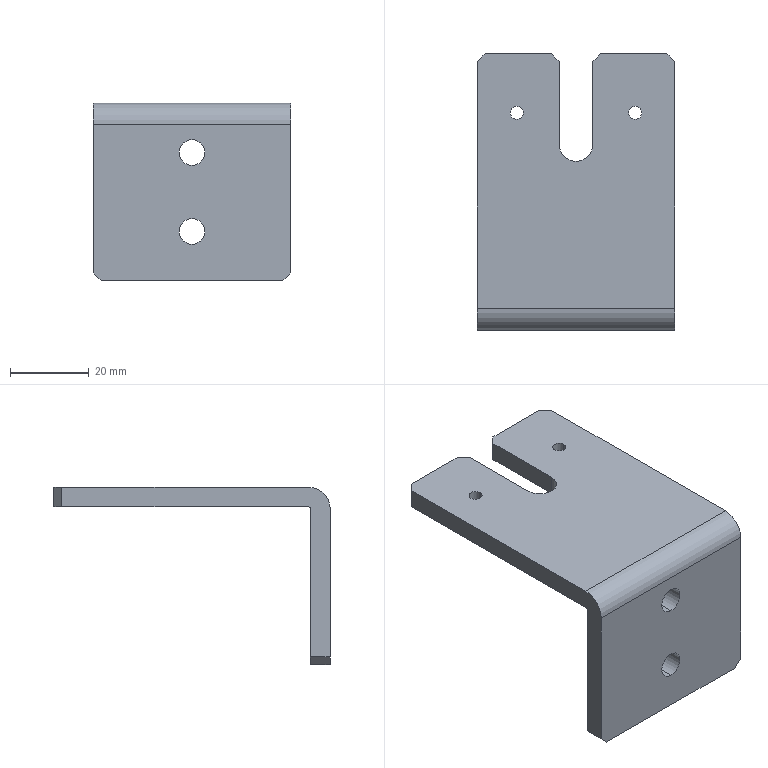Part | SolidWorks | features BaseBody 1 | 1 solid | 28 faces | box 50 x 70 x 45 mm | volume 25581 mm3 | plane 17 | cylinder 11 | commonest cylinder face diameters 3.3 x4 6.5 x4 1 x1 8.5 x1 11 x1
STEP:
#1=CARTESIAN_POINT('',(13.35,55.,-5.));
#2=VERTEX_POINT('',#1);
#3=CARTESIAN_POINT('',(16.65,55.,-5.));
#4=VERTEX_POINT('',#3);
#5=CARTESIAN_POINT('',(15.,55.,-5.));
#6=DIRECTION('',(0.,0.,1.));
#7=DIRECTION('',(1.,0.,0.));
#8=AXIS2_PLACEMENT_3D('',#5,#6,#7);
#9=CIRCLE('',#8,1.65);
#10=EDGE_CURVE('',#2,#4,#9,.T.);
#11=ORIENTED_EDGE('',*,*,#10,.F.);
#12=CARTESIAN_POINT('',(13.35,55.,0.));
#13=VERTEX_POINT('',#12);
#14=CARTESIAN_POINT('',(13.35,55.,0.));
#15=DIRECTION('',(0.,0.,1.));
#16=VECTOR('',#15,1000.);
#17=LINE('',#14,#16);
#18=EDGE_CURVE('',#2,#13,#17,.T.);
#19=ORIENTED_EDGE('',*,*,#18,.T.);
#20=CARTESIAN_POINT('',(16.65,55.,0.));
#21=VERTEX_POINT('',#20);
#22=CARTESIAN_POINT('',(15.,55.,0.));
#23=DIRECTION('',(0.,0.,-1.));
#24=DIRECTION('',(1.,0.,0.));
#25=AXIS2_PLACEMENT_3D('',#22,#23,#24);
#26=CIRCLE('',#25,1.65);
#27=EDGE_CURVE('',#21,#13,#26,.T.);
#28=ORIENTED_EDGE('',*,*,#27,.F.);
#29=CARTESIAN_POINT('',(16.65,55.,0.));
#30=DIRECTION('',(0.,0.,1.));
#31=VECTOR('',#30,1000.);
#32=LINE('',#29,#31);
#33=EDGE_CURVE('',#4,#21,#32,.T.);
#34=ORIENTED_EDGE('',*,*,#33,.F.);
#35=EDGE_LOOP('',(#11,#19,#28,#34));
#36=FACE_OUTER_BOUND('',#35,.T.);
#37=CARTESIAN_POINT('',(15.,55.,0.));
#38=DIRECTION('',(0.,0.,1.));
#39=DIRECTION('',(1.,0.,0.));
#40=AXIS2_PLACEMENT_3D('',#37,#38,#39);
#41=CYLINDRICAL_SURFACE('',#40,1.65);
#42=ADVANCED_FACE('',(#36),#41,.F.);
#43=CARTESIAN_POINT('',(-16.65,55.,-5.));
#44=VERTEX_POINT('',#43);
#45=CARTESIAN_POINT('',(-13.35,55.,-5.));
#46=VERTEX_POINT('',#45);
#47=CARTESIAN_POINT('',(-15.,55.,-5.));
#48=DIRECTION('',(0.,0.,1.));
#49=DIRECTION('',(1.,0.,0.));
#50=AXIS2_PLACEMENT_3D('',#47,#48,#49);
#51=CIRCLE('',#50,1.65);
#52=EDGE_CURVE('',#44,#46,#51,.T.);
#53=ORIENTED_EDGE('',*,*,#52,.F.);
#54=CARTESIAN_POINT('',(-16.65,55.,0.));
#55=VERTEX_POINT('',#54);
#56=CARTESIAN_POINT('',(-16.65,55.,0.));
#57=DIRECTION('',(0.,0.,1.));
#58=VECTOR('',#57,1000.);
#59=LINE('',#56,#58);
#60=EDGE_CURVE('',#44,#55,#59,.T.);
#61=ORIENTED_EDGE('',*,*,#60,.T.);
#62=CARTESIAN_POINT('',(-13.35,55.,0.));
#63=VERTEX_POINT('',#62);
#64=CARTESIAN_POINT('',(-15.,55.,0.));
#65=DIRECTION('',(0.,0.,-1.));
#66=DIRECTION('',(1.,0.,0.));
#67=AXIS2_PLACEMENT_3D('',#64,#65,#66);
#68=CIRCLE('',#67,1.65);
#69=EDGE_CURVE('',#63,#55,#68,.T.);
#70=ORIENTED_EDGE('',*,*,#69,.F.);
#71=CARTESIAN_POINT('',(-13.35,55.,0.));
#72=DIRECTION('',(0.,0.,1.));
#73=VECTOR('',#72,1000.);
#74=LINE('',#71,#73);
#75=EDGE_CURVE('',#46,#63,#74,.T.);
#76=ORIENTED_EDGE('',*,*,#75,.F.);
#77=EDGE_LOOP('',(#53,#61,#70,#76));
#78=FACE_OUTER_BOUND('',#77,.T.);
#79=CARTESIAN_POINT('',(-15.,55.,0.));
#80=DIRECTION('',(0.,0.,1.));
#81=DIRECTION('',(1.,0.,0.));
#82=AXIS2_PLACEMENT_3D('',#79,#80,#81);
#83=CYLINDRICAL_SURFACE('',#82,1.65);
#84=ADVANCED_FACE('',(#78),#83,.F.);
#85=CARTESIAN_POINT('',(0.,5.,-29.25));
#86=VERTEX_POINT('',#85);
#87=CARTESIAN_POINT('',(0.,5.,-35.75));
#88=VERTEX_POINT('',#87);
#89=CARTESIAN_POINT('',(0.,5.,-32.5));
#90=DIRECTION('',(0.,-1.,0.));
#91=DIRECTION('',(0.,0.,-1.));
#92=AXIS2_PLACEMENT_3D('',#89,#90,#91);
#93=CIRCLE('',#92,3.25);
#94=EDGE_CURVE('',#86,#88,#93,.T.);
#95=ORIENTED_EDGE('',*,*,#94,.F.);
#96=CARTESIAN_POINT('',(0.,0.,-29.25));
#97=VERTEX_POINT('',#96);
#98=CARTESIAN_POINT('',(0.,0.,-29.25));
#99=DIRECTION('',(0.,-1.,0.));
#100=VECTOR('',#99,1000.);
#101=LINE('',#98,#100);
#102=EDGE_CURVE('',#86,#97,#101,.T.);
#103=ORIENTED_EDGE('',*,*,#102,.T.);
#104=CARTESIAN_POINT('',(0.,0.,-35.75));
#105=VERTEX_POINT('',#104);
#106=CARTESIAN_POINT('',(0.,0.,-32.5));
#107=DIRECTION('',(0.,1.,0.));
#108=DIRECTION('',(0.,0.,-1.));
#109=AXIS2_PLACEMENT_3D('',#106,#107,#108);
#110=CIRCLE('',#109,3.25);
#111=EDGE_CURVE('',#105,#97,#110,.T.);
#112=ORIENTED_EDGE('',*,*,#111,.F.);
#113=CARTESIAN_POINT('',(0.,0.,-35.75));
#114=DIRECTION('',(0.,-1.,0.));
#115=VECTOR('',#114,1000.);
#116=LINE('',#113,#115);
#117=EDGE_CURVE('',#88,#105,#116,.T.);
#118=ORIENTED_EDGE('',*,*,#117,.F.);
#119=EDGE_LOOP('',(#95,#103,#112,#118));
#120=FACE_OUTER_BOUND('',#119,.T.);
#121=CARTESIAN_POINT('',(0.,0.,-32.5));
#122=DIRECTION('',(0.,-1.,0.));
#123=DIRECTION('',(0.,0.,-1.));
#124=AXIS2_PLACEMENT_3D('',#121,#122,#123);
#125=CYLINDRICAL_SURFACE('',#124,3.25);
#126=ADVANCED_FACE('',(#120),#125,.F.);
#127=CARTESIAN_POINT('',(0.,5.,-9.25));
#128=VERTEX_POINT('',#127);
#129=CARTESIAN_POINT('',(0.,5.,-15.75));
#130=VERTEX_POINT('',#129);
#131=CARTESIAN_POINT('',(0.,5.,-12.5));
#132=DIRECTION('',(0.,-1.,0.));
#133=DIRECTION('',(0.,0.,-1.));
#134=AXIS2_PLACEMENT_3D('',#131,#132,#133);
#135=CIRCLE('',#134,3.25);
#136=EDGE_CURVE('',#128,#130,#135,.T.);
#137=ORIENTED_EDGE('',*,*,#136,.F.);
#138=CARTESIAN_POINT('',(0.,0.,-9.25));
#139=VERTEX_POINT('',#138);
#140=CARTESIAN_POINT('',(0.,0.,-9.25));
#141=DIRECTION('',(0.,-1.,0.));
#142=VECTOR('',#141,1000.);
#143=LINE('',#140,#142);
#144=EDGE_CURVE('',#128,#139,#143,.T.);
#145=ORIENTED_EDGE('',*,*,#144,.T.);
#146=CARTESIAN_POINT('',(0.,0.,-15.75));
#147=VERTEX_POINT('',#146);
#148=CARTESIAN_POINT('',(0.,0.,-12.5));
#149=DIRECTION('',(0.,1.,0.));
#150=DIRECTION('',(0.,0.,-1.));
#151=AXIS2_PLACEMENT_3D('',#148,#149,#150);
#152=CIRCLE('',#151,3.25);
#153=EDGE_CURVE('',#147,#139,#152,.T.);
#154=ORIENTED_EDGE('',*,*,#153,.F.);
#155=CARTESIAN_POINT('',(0.,0.,-15.75));
#156=DIRECTION('',(0.,-1.,0.));
#157=VECTOR('',#156,1000.);
#158=LINE('',#155,#157);
#159=EDGE_CURVE('',#130,#147,#158,.T.);
#160=ORIENTED_EDGE('',*,*,#159,.F.);
#161=EDGE_LOOP('',(#137,#145,#154,#160));
#162=FACE_OUTER_BOUND('',#161,.T.);
#163=CARTESIAN_POINT('',(0.,0.,-12.5));
#164=DIRECTION('',(0.,-1.,0.));
#165=DIRECTION('',(0.,0.,-1.));
#166=AXIS2_PLACEMENT_3D('',#163,#164,#165);
#167=CYLINDRICAL_SURFACE('',#166,3.25);
#168=ADVANCED_FACE('',(#162),#167,.F.);
#169=CARTESIAN_POINT('',(15.,55.,-5.));
#170=DIRECTION('',(0.,0.,1.));
#171=DIRECTION('',(1.,0.,0.));
#172=AXIS2_PLACEMENT_3D('',#169,#170,#171);
#173=CIRCLE('',#172,1.65);
#174=EDGE_CURVE('',#4,#2,#173,.T.);
#175=ORIENTED_EDGE('',*,*,#174,.T.);
#176=ORIENTED_EDGE('',*,*,#10,.T.);
#177=EDGE_LOOP('',(#175,#176));
#178=FACE_BOUND('',#177,.T.);
#179=CARTESIAN_POINT('',(-15.,55.,-5.));
#180=DIRECTION('',(0.,0.,1.));
#181=DIRECTION('',(1.,0.,0.));
#182=AXIS2_PLACEMENT_3D('',#179,#180,#181);
#183=CIRCLE('',#182,1.65);
#184=EDGE_CURVE('',#46,#44,#183,.T.);
#185=ORIENTED_EDGE('',*,*,#184,.T.);
#186=ORIENTED_EDGE('',*,*,#52,.T.);
#187=EDGE_LOOP('',(#185,#186));
#188=FACE_BOUND('',#187,.T.);
#189=CARTESIAN_POINT('',(4.25,47.,-5.));
#190=VERTEX_POINT('',#189);
#191=CARTESIAN_POINT('',(4.25,68.,-5.));
#192=VERTEX_POINT('',#191);
#193=CARTESIAN_POINT('',(4.25,0.,-5.));
#194=DIRECTION('',(0.,1.,0.));
#195=VECTOR('',#194,1000.);
#196=LINE('',#193,#195);
#197=EDGE_CURVE('',#190,#192,#196,.T.);
#198=ORIENTED_EDGE('',*,*,#197,.T.);
#199=CARTESIAN_POINT('',(6.25,70.,-5.));
#200=VERTEX_POINT('',#199);
#201=CARTESIAN_POINT('',(4.25,68.,-5.));
#202=DIRECTION('',(0.7071,0.7071,0.));
#203=VECTOR('',#202,1000.);
#204=LINE('',#201,#203);
#205=EDGE_CURVE('',#192,#200,#204,.T.);
#206=ORIENTED_EDGE('',*,*,#205,.T.);
#207=CARTESIAN_POINT('',(23.,70.,-5.));
#208=VERTEX_POINT('',#207);
#209=CARTESIAN_POINT('',(-25.,70.,-5.));
#210=DIRECTION('',(1.,0.,0.));
#211=VECTOR('',#210,1000.);
#212=LINE('',#209,#211);
#213=EDGE_CURVE('',#200,#208,#212,.T.);
#214=ORIENTED_EDGE('',*,*,#213,.T.);
#215=CARTESIAN_POINT('',(25.,68.,-5.));
#216=VERTEX_POINT('',#215);
#217=CARTESIAN_POINT('',(23.,70.,-5.));
#218=DIRECTION('',(0.7071,-0.7071,0.));
#219=VECTOR('',#218,1000.);
#220=LINE('',#217,#219);
#221=EDGE_CURVE('',#208,#216,#220,.T.);
#222=ORIENTED_EDGE('',*,*,#221,.T.);
#223=CARTESIAN_POINT('',(25.,5.5,-5.));
#224=VERTEX_POINT('',#223);
#225=CARTESIAN_POINT('',(25.,0.,-5.));
#226=DIRECTION('',(0.,-1.,0.));
#227=VECTOR('',#226,1000.);
#228=LINE('',#225,#227);
#229=EDGE_CURVE('',#216,#224,#228,.T.);
#230=ORIENTED_EDGE('',*,*,#229,.T.);
#231=CARTESIAN_POINT('',(-25.,5.5,-5.));
#232=VERTEX_POINT('',#231);
#233=CARTESIAN_POINT('',(-25.,5.5,-5.));
#234=DIRECTION('',(-1.,0.,0.));
#235=VECTOR('',#234,1000.);
#236=LINE('',#233,#235);
#237=EDGE_CURVE('',#224,#232,#236,.T.);
#238=ORIENTED_EDGE('',*,*,#237,.T.);
#239=CARTESIAN_POINT('',(-25.,68.,-5.));
#240=VERTEX_POINT('',#239);
#241=CARTESIAN_POINT('',(-25.,0.,-5.));
#242=DIRECTION('',(0.,1.,0.));
#243=VECTOR('',#242,1000.);
#244=LINE('',#241,#243);
#245=EDGE_CURVE('',#232,#240,#244,.T.);
#246=ORIENTED_EDGE('',*,*,#245,.T.);
#247=CARTESIAN_POINT('',(-23.,70.,-5.));
#248=VERTEX_POINT('',#247);
#249=CARTESIAN_POINT('',(-25.,68.,-5.));
#250=DIRECTION('',(0.7071,0.7071,0.));
#251=VECTOR('',#250,1000.);
#252=LINE('',#249,#251);
#253=EDGE_CURVE('',#240,#248,#252,.T.);
#254=ORIENTED_EDGE('',*,*,#253,.T.);
#255=CARTESIAN_POINT('',(-6.25,70.,-5.));
#256=VERTEX_POINT('',#255);
#257=CARTESIAN_POINT('',(-25.,70.,-5.));
#258=DIRECTION('',(1.,0.,0.));
#259=VECTOR('',#258,1000.);
#260=LINE('',#257,#259);
#261=EDGE_CURVE('',#248,#256,#260,.T.);
#262=ORIENTED_EDGE('',*,*,#261,.T.);
#263=CARTESIAN_POINT('',(-4.25,68.,-5.));
#264=VERTEX_POINT('',#263);
#265=CARTESIAN_POINT('',(-6.25,70.,-5.));
#266=DIRECTION('',(0.7071,-0.7071,0.));
#267=VECTOR('',#266,1000.);
#268=LINE('',#265,#267);
#269=EDGE_CURVE('',#256,#264,#268,.T.);
#270=ORIENTED_EDGE('',*,*,#269,.T.);
#271=CARTESIAN_POINT('',(-4.25,47.,-5.));
#272=VERTEX_POINT('',#271);
#273=CARTESIAN_POINT('',(-4.25,0.,-5.));
#274=DIRECTION('',(0.,-1.,0.));
#275=VECTOR('',#274,1000.);
#276=LINE('',#273,#275);
#277=EDGE_CURVE('',#264,#272,#276,.T.);
#278=ORIENTED_EDGE('',*,*,#277,.T.);
#279=CARTESIAN_POINT('',(0.,47.,-5.));
#280=DIRECTION('',(0.,0.,1.));
#281=DIRECTION('',(1.,0.,0.));
#282=AXIS2_PLACEMENT_3D('',#279,#280,#281);
#283=CIRCLE('',#282,4.25);
#284=EDGE_CURVE('',#272,#190,#283,.T.);
#285=ORIENTED_EDGE('',*,*,#284,.T.);
#286=EDGE_LOOP('',(#198,#206,#214,#222,#230,#238,#246,#254,#262,#270,#278,#285));
#287=FACE_OUTER_BOUND('',#286,.T.);
#288=CARTESIAN_POINT('',(-25.,0.,-5.));
#289=DIRECTION('',(0.,0.,-1.));
#290=DIRECTION('',(-1.,0.,0.));
#291=AXIS2_PLACEMENT_3D('',#288,#289,#290);
#292=PLANE('',#291);
#293=ADVANCED_FACE('',(#178,#188,#287),#292,.T.);
#294=ORIENTED_EDGE('',*,*,#18,.F.);
#295=ORIENTED_EDGE('',*,*,#174,.F.);
#296=ORIENTED_EDGE('',*,*,#33,.T.);
#297=CARTESIAN_POINT('',(15.,55.,0.));
#298=DIRECTION('',(0.,0.,-1.));
#299=DIRECTION('',(1.,0.,0.));
#300=AXIS2_PLACEMENT_3D('',#297,#298,#299);
#301=CIRCLE('',#300,1.65);
#302=EDGE_CURVE('',#13,#21,#301,.T.);
#303=ORIENTED_EDGE('',*,*,#302,.F.);
#304=EDGE_LOOP('',(#294,#295,#296,#303));
#305=FACE_OUTER_BOUND('',#304,.T.);
#306=CARTESIAN_POINT('',(15.,55.,0.));
#307=DIRECTION('',(0.,0.,1.));
#308=DIRECTION('',(1.,0.,0.));
#309=AXIS2_PLACEMENT_3D('',#306,#307,#308);
#310=CYLINDRICAL_SURFACE('',#309,1.65);
#311=ADVANCED_FACE('',(#305),#310,.F.);
#312=ORIENTED_EDGE('',*,*,#60,.F.);
#313=ORIENTED_EDGE('',*,*,#184,.F.);
#314=ORIENTED_EDGE('',*,*,#75,.T.);
#315=CARTESIAN_POINT('',(-15.,55.,0.));
#316=DIRECTION('',(0.,0.,-1.));
#317=DIRECTION('',(1.,0.,0.));
#318=AXIS2_PLACEMENT_3D('',#315,#316,#317);
#319=CIRCLE('',#318,1.65);
#320=EDGE_CURVE('',#55,#63,#319,.T.);
#321=ORIENTED_EDGE('',*,*,#320,.F.);
#322=EDGE_LOOP('',(#312,#313,#314,#321));
#323=FACE_OUTER_BOUND('',#322,.T.);
#324=CARTESIAN_POINT('',(-15.,55.,0.));
#325=DIRECTION('',(0.,0.,1.));
#326=DIRECTION('',(1.,0.,0.));
#327=AXIS2_PLACEMENT_3D('',#324,#325,#326);
#328=CYLINDRICAL_SURFACE('',#327,1.65);
#329=ADVANCED_FACE('',(#323),#328,.F.);
#330=CARTESIAN_POINT('',(4.25,68.,0.));
#331=VERTEX_POINT('',#330);
#332=CARTESIAN_POINT('',(4.25,68.,0.));
#333=DIRECTION('',(0.,0.,-1.));
#334=VECTOR('',#333,1000.);
#335=LINE('',#332,#334);
#336=EDGE_CURVE('',#331,#192,#335,.T.);
#337=ORIENTED_EDGE('',*,*,#336,.F.);
#338=CARTESIAN_POINT('',(6.25,70.,0.));
#339=VERTEX_POINT('',#338);
#340=CARTESIAN_POINT('',(6.25,70.,0.));
#341=DIRECTION('',(-0.7071,-0.7071,0.));
#342=VECTOR('',#341,1000.);
#343=LINE('',#340,#342);
#344=EDGE_CURVE('',#339,#331,#343,.T.);
#345=ORIENTED_EDGE('',*,*,#344,.F.);
#346=CARTESIAN_POINT('',(6.25,70.,0.));
#347=DIRECTION('',(0.,0.,1.));
#348=VECTOR('',#347,1000.);
#349=LINE('',#346,#348);
#350=EDGE_CURVE('',#200,#339,#349,.T.);
#351=ORIENTED_EDGE('',*,*,#350,.F.);
#352=ORIENTED_EDGE('',*,*,#205,.F.);
#353=EDGE_LOOP('',(#337,#345,#351,#352));
#354=FACE_OUTER_BOUND('',#353,.T.);
#355=CARTESIAN_POINT('',(6.25,70.,0.));
#356=DIRECTION('',(0.7071,-0.7071,0.));
#357=DIRECTION('',(0.7071,0.7071,0.));
#358=AXIS2_PLACEMENT_3D('',#355,#356,#357);
#359=PLANE('',#358);
#360=ADVANCED_FACE('',(#354),#359,.F.);
#361=ORIENTED_EDGE('',*,*,#336,.T.);
#362=ORIENTED_EDGE('',*,*,#197,.F.);
#363=CARTESIAN_POINT('',(4.25,47.,0.));
#364=VERTEX_POINT('',#363);
#365=CARTESIAN_POINT('',(4.25,47.,-45.));
#366=DIRECTION('',(0.,0.,-1.));
#367=VECTOR('',#366,1000.);
#368=LINE('',#365,#367);
#369=EDGE_CURVE('',#364,#190,#368,.T.);
#370=ORIENTED_EDGE('',*,*,#369,.F.);
#371=CARTESIAN_POINT('',(4.25,93.,0.));
#372=DIRECTION('',(0.,-1.,0.));
#373=VECTOR('',#372,1000.);
#374=LINE('',#371,#373);
#375=EDGE_CURVE('',#331,#364,#374,.T.);
#376=ORIENTED_EDGE('',*,*,#375,.F.);
#377=EDGE_LOOP('',(#361,#362,#370,#376));
#378=FACE_OUTER_BOUND('',#377,.T.);
#379=CARTESIAN_POINT('',(4.25,93.,-45.));
#380=DIRECTION('',(1.,0.,0.));
#381=DIRECTION('',(0.,1.,0.));
#382=AXIS2_PLACEMENT_3D('',#379,#380,#381);
#383=PLANE('',#382);
#384=ADVANCED_FACE('',(#378),#383,.F.);
#385=CARTESIAN_POINT('',(-4.25,47.,0.));
#386=VERTEX_POINT('',#385);
#387=CARTESIAN_POINT('',(-4.25,47.,-45.));
#388=DIRECTION('',(0.,0.,-1.));
#389=VECTOR('',#388,1000.);
#390=LINE('',#387,#389);
#391=EDGE_CURVE('',#386,#272,#390,.T.);
#392=ORIENTED_EDGE('',*,*,#391,.F.);
#393=CARTESIAN_POINT('',(0.,47.,0.));
#394=DIRECTION('',(0.,0.,-1.));
#395=DIRECTION('',(1.,0.,0.));
#396=AXIS2_PLACEMENT_3D('',#393,#394,#395);
#397=CIRCLE('',#396,4.25);
#398=EDGE_CURVE('',#364,#386,#397,.T.);
#399=ORIENTED_EDGE('',*,*,#398,.F.);
#400=ORIENTED_EDGE('',*,*,#369,.T.);
#401=ORIENTED_EDGE('',*,*,#284,.F.);
#402=EDGE_LOOP('',(#392,#399,#400,#401));
#403=FACE_OUTER_BOUND('',#402,.T.);
#404=CARTESIAN_POINT('',(0.,47.,-45.));
#405=DIRECTION('',(0.,0.,1.));
#406=DIRECTION('',(1.,0.,0.));
#407=AXIS2_PLACEMENT_3D('',#404,#405,#406);
#408=CYLINDRICAL_SURFACE('',#407,4.25);
#409=ADVANCED_FACE('',(#403),#408,.F.);
#410=CARTESIAN_POINT('',(-4.25,68.,0.));
#411=VERTEX_POINT('',#410);
#412=CARTESIAN_POINT('',(-4.25,68.,-45.));
#413=DIRECTION('',(0.,0.,-1.));
#414=VECTOR('',#413,1000.);
#415=LINE('',#412,#414);
#416=EDGE_CURVE('',#411,#264,#415,.T.);
#417=ORIENTED_EDGE('',*,*,#416,.F.);
#418=CARTESIAN_POINT('',(-4.25,93.,0.));
#419=DIRECTION('',(0.,1.,0.));
#420=VECTOR('',#419,1000.);
#421=LINE('',#418,#420);
#422=EDGE_CURVE('',#386,#411,#421,.T.);
#423=ORIENTED_EDGE('',*,*,#422,.F.);
#424=ORIENTED_EDGE('',*,*,#391,.T.);
#425=ORIENTED_EDGE('',*,*,#277,.F.);
#426=EDGE_LOOP('',(#417,#423,#424,#425));
#427=FACE_OUTER_BOUND('',#426,.T.);
#428=CARTESIAN_POINT('',(-4.25,93.,-45.));
#429=DIRECTION('',(-1.,0.,0.));
#430=DIRECTION('',(0.,-1.,0.));
#431=AXIS2_PLACEMENT_3D('',#428,#429,#430);
#432=PLANE('',#431);
#433=ADVANCED_FACE('',(#427),#432,.F.);
#434=ORIENTED_EDGE('',*,*,#416,.T.);
#435=ORIENTED_EDGE('',*,*,#269,.F.);
#436=CARTESIAN_POINT('',(-6.25,70.,0.));
#437=VERTEX_POINT('',#436);
#438=CARTESIAN_POINT('',(-6.25,70.,0.));
#439=DIRECTION('',(0.,0.,-1.));
#440=VECTOR('',#439,1000.);
#441=LINE('',#438,#440);
#442=EDGE_CURVE('',#437,#256,#441,.T.);
#443=ORIENTED_EDGE('',*,*,#442,.F.);
#444=CARTESIAN_POINT('',(-6.25,70.,0.));
#445=DIRECTION('',(-0.7071,0.7071,0.));
#446=VECTOR('',#445,1000.);
#447=LINE('',#444,#446);
#448=EDGE_CURVE('',#411,#437,#447,.T.);
#449=ORIENTED_EDGE('',*,*,#448,.F.);
#450=EDGE_LOOP('',(#434,#435,#443,#449));
#451=FACE_OUTER_BOUND('',#450,.T.);
#452=CARTESIAN_POINT('',(-6.25,70.,0.));
#453=DIRECTION('',(-0.7071,-0.7071,0.));
#454=DIRECTION('',(0.7071,-0.7071,0.));
#455=AXIS2_PLACEMENT_3D('',#452,#453,#454);
#456=PLANE('',#455);
#457=ADVANCED_FACE('',(#451),#456,.F.);
#458=ORIENTED_EDGE('',*,*,#442,.T.);
#459=ORIENTED_EDGE('',*,*,#261,.F.);
#460=CARTESIAN_POINT('',(-23.,70.,0.));
#461=VERTEX_POINT('',#460);
#462=CARTESIAN_POINT('',(-23.,70.,0.));
#463=DIRECTION('',(0.,0.,-1.));
#464=VECTOR('',#463,1000.);
#465=LINE('',#462,#464);
#466=EDGE_CURVE('',#461,#248,#465,.T.);
#467=ORIENTED_EDGE('',*,*,#466,.F.);
#468=CARTESIAN_POINT('',(-25.,70.,0.));
#469=DIRECTION('',(-1.,0.,0.));
#470=VECTOR('',#469,1000.);
#471=LINE('',#468,#470);
#472=EDGE_CURVE('',#437,#461,#471,.T.);
#473=ORIENTED_EDGE('',*,*,#472,.F.);
#474=EDGE_LOOP('',(#458,#459,#467,#473));
#475=FACE_OUTER_BOUND('',#474,.T.);
#476=CARTESIAN_POINT('',(-25.,70.,0.));
#477=DIRECTION('',(0.,-1.,0.));
#478=DIRECTION('',(0.,0.,-1.));
#479=AXIS2_PLACEMENT_3D('',#476,#477,#478);
#480=PLANE('',#479);
#481=ADVANCED_FACE('',(#475),#480,.F.);
#482=ORIENTED_EDGE('',*,*,#466,.T.);
#483=ORIENTED_EDGE('',*,*,#253,.F.);
#484=CARTESIAN_POINT('',(-25.,68.,0.));
#485=VERTEX_POINT('',#484);
#486=CARTESIAN_POINT('',(-25.,68.,-5.5));
#487=DIRECTION('',(0.,0.,-1.));
#488=VECTOR('',#487,1000.);
#489=LINE('',#486,#488);
#490=EDGE_CURVE('',#485,#240,#489,.T.);
#491=ORIENTED_EDGE('',*,*,#490,.F.);
#492=CARTESIAN_POINT('',(-25.,68.,0.));
#493=DIRECTION('',(-0.7071,-0.7071,0.));
#494=VECTOR('',#493,1000.);
#495=LINE('',#492,#494);
#496=EDGE_CURVE('',#461,#485,#495,.T.);
#497=ORIENTED_EDGE('',*,*,#496,.F.);
#498=EDGE_LOOP('',(#482,#483,#491,#497));
#499=FACE_OUTER_BOUND('',#498,.T.);
#500=CARTESIAN_POINT('',(-25.,68.,-5.5));
#501=DIRECTION('',(0.7071,-0.7071,0.));
#502=DIRECTION('',(0.7071,0.7071,0.));
#503=AXIS2_PLACEMENT_3D('',#500,#501,#502);
#504=PLANE('',#503);
#505=ADVANCED_FACE('',(#499),#504,.F.);
#506=ORIENTED_EDGE('',*,*,#490,.T.);
#507=ORIENTED_EDGE('',*,*,#245,.F.);
#508=CARTESIAN_POINT('',(-25.,5.,-5.5));
#509=VERTEX_POINT('',#508);
#510=CARTESIAN_POINT('',(-25.,5.5,-5.5));
#511=DIRECTION('',(1.,0.,0.));
#512=DIRECTION('',(0.,0.,-1.));
#513=AXIS2_PLACEMENT_3D('',#510,#511,#512);
#514=CIRCLE('',#513,0.5);
#515=EDGE_CURVE('',#232,#509,#514,.T.);
#516=ORIENTED_EDGE('',*,*,#515,.T.);
#517=CARTESIAN_POINT('',(-25.,5.,-43.));
#518=VERTEX_POINT('',#517);
#519=CARTESIAN_POINT('',(-25.,5.,-45.));
#520=DIRECTION('',(0.,0.,1.));
#521=VECTOR('',#520,1000.);
#522=LINE('',#519,#521);
#523=EDGE_CURVE('',#518,#509,#522,.T.);
#524=ORIENTED_EDGE('',*,*,#523,.F.);
#525=CARTESIAN_POINT('',(-25.,0.,-43.));
#526=VERTEX_POINT('',#525);
#527=CARTESIAN_POINT('',(-25.,5.5,-43.));
#528=DIRECTION('',(0.,-1.,0.));
#529=VECTOR('',#528,1000.);
#530=LINE('',#527,#529);
#531=EDGE_CURVE('',#518,#526,#530,.T.);
#532=ORIENTED_EDGE('',*,*,#531,.T.);
#533=CARTESIAN_POINT('',(-25.,0.,-5.5));
#534=VERTEX_POINT('',#533);
#535=CARTESIAN_POINT('',(-25.,0.,-5.));
#536=DIRECTION('',(0.,0.,1.));
#537=VECTOR('',#536,1000.);
#538=LINE('',#535,#537);
#539=EDGE_CURVE('',#526,#534,#538,.T.);
#540=ORIENTED_EDGE('',*,*,#539,.T.);
#541=CARTESIAN_POINT('',(-25.,5.5,0.));
#542=VERTEX_POINT('',#541);
#543=CARTESIAN_POINT('',(-25.,5.5,-5.5));
#544=DIRECTION('',(-1.,0.,0.));
#545=DIRECTION('',(0.,0.,-1.));
#546=AXIS2_PLACEMENT_3D('',#543,#544,#545);
#547=CIRCLE('',#546,5.5);
#548=EDGE_CURVE('',#534,#542,#547,.T.);
#549=ORIENTED_EDGE('',*,*,#548,.T.);
#550=CARTESIAN_POINT('',(-25.,5.5,0.));
#551=DIRECTION('',(0.,-1.,0.));
#552=VECTOR('',#551,1000.);
#553=LINE('',#550,#552);
#554=EDGE_CURVE('',#485,#542,#553,.T.);
#555=ORIENTED_EDGE('',*,*,#554,.F.);
#556=EDGE_LOOP('',(#506,#507,#516,#524,#532,#540,#549,#555));
#557=FACE_OUTER_BOUND('',#556,.T.);
#558=CARTESIAN_POINT('',(-25.,5.5,-5.5));
#559=DIRECTION('',(1.,0.,0.));
#560=DIRECTION('',(0.,0.,-1.));
#561=AXIS2_PLACEMENT_3D('',#558,#559,#560);
#562=PLANE('',#561);
#563=ADVANCED_FACE('',(#557),#562,.F.);
#564=CARTESIAN_POINT('',(25.,5.,-5.5));
#565=VERTEX_POINT('',#564);
#566=CARTESIAN_POINT('',(-25.,5.,-5.5));
#567=DIRECTION('',(1.,0.,0.));
#568=VECTOR('',#567,1000.);
#569=LINE('',#566,#568);
#570=EDGE_CURVE('',#509,#565,#569,.T.);
#571=ORIENTED_EDGE('',*,*,#570,.F.);
#572=ORIENTED_EDGE('',*,*,#515,.F.);
#573=ORIENTED_EDGE('',*,*,#237,.F.);
#574=CARTESIAN_POINT('',(25.,5.5,-5.5));
#575=DIRECTION('',(-1.,0.,0.));
#576=DIRECTION('',(0.,0.,-1.));
#577=AXIS2_PLACEMENT_3D('',#574,#575,#576);
#578=CIRCLE('',#577,0.5);
#579=EDGE_CURVE('',#565,#224,#578,.T.);
#580=ORIENTED_EDGE('',*,*,#579,.F.);
#581=EDGE_LOOP('',(#571,#572,#573,#580));
#582=FACE_OUTER_BOUND('',#581,.T.);
#583=CARTESIAN_POINT('',(-25.,5.5,-5.5));
#584=DIRECTION('',(1.,0.,0.));
#585=DIRECTION('',(0.,0.,-1.));
#586=AXIS2_PLACEMENT_3D('',#583,#584,#585);
#587=CYLINDRICAL_SURFACE('',#586,0.5);
#588=ADVANCED_FACE('',(#582),#587,.F.);
#589=CARTESIAN_POINT('',(25.,68.,0.));
#590=VERTEX_POINT('',#589);
#591=CARTESIAN_POINT('',(25.,5.5,0.));
#592=VERTEX_POINT('',#591);
#593=CARTESIAN_POINT('',(25.,5.,0.));
#594=DIRECTION('',(0.,-1.,0.));
#595=VECTOR('',#594,1000.);
#596=LINE('',#593,#595);
#597=EDGE_CURVE('',#590,#592,#596,.T.);
#598=ORIENTED_EDGE('',*,*,#597,.T.);
#599=CARTESIAN_POINT('',(25.,0.,-5.5));
#600=VERTEX_POINT('',#599);
#601=CARTESIAN_POINT('',(25.,5.5,-5.5));
#602=DIRECTION('',(1.,0.,0.));
#603=DIRECTION('',(0.,0.,-1.));
#604=AXIS2_PLACEMENT_3D('',#601,#602,#603);
#605=CIRCLE('',#604,5.5);
#606=EDGE_CURVE('',#592,#600,#605,.T.);
#607=ORIENTED_EDGE('',*,*,#606,.T.);
#608=CARTESIAN_POINT('',(25.,0.,-43.));
#609=VERTEX_POINT('',#608);
#610=CARTESIAN_POINT('',(25.,0.,-5.5));
#611=DIRECTION('',(0.,0.,-1.));
#612=VECTOR('',#611,1000.);
#613=LINE('',#610,#612);
#614=EDGE_CURVE('',#600,#609,#613,.T.);
#615=ORIENTED_EDGE('',*,*,#614,.T.);
#616=CARTESIAN_POINT('',(25.,5.,-43.));
#617=VERTEX_POINT('',#616);
#618=CARTESIAN_POINT('',(25.,5.,-43.));
#619=DIRECTION('',(0.,-1.,0.));
#620=VECTOR('',#619,1000.);
#621=LINE('',#618,#620);
#622=EDGE_CURVE('',#617,#609,#621,.T.);
#623=ORIENTED_EDGE('',*,*,#622,.F.);
#624=CARTESIAN_POINT('',(25.,5.,-45.));
#625=DIRECTION('',(0.,0.,-1.));
#626=VECTOR('',#625,1000.);
#627=LINE('',#624,#626);
#628=EDGE_CURVE('',#565,#617,#627,.T.);
#629=ORIENTED_EDGE('',*,*,#628,.F.);
#630=ORIENTED_EDGE('',*,*,#579,.T.);
#631=ORIENTED_EDGE('',*,*,#229,.F.);
#632=CARTESIAN_POINT('',(25.,68.,-5.5));
#633=DIRECTION('',(0.,0.,1.));
#634=VECTOR('',#633,1000.);
#635=LINE('',#632,#634);
#636=EDGE_CURVE('',#216,#590,#635,.T.);
#637=ORIENTED_EDGE('',*,*,#636,.T.);
#638=EDGE_LOOP('',(#598,#607,#615,#623,#629,#630,#631,#637));
#639=FACE_OUTER_BOUND('',#638,.T.);
#640=CARTESIAN_POINT('',(25.,5.,-5.5));
#641=DIRECTION('',(1.,0.,0.));
#642=DIRECTION('',(0.,0.,-1.));
#643=AXIS2_PLACEMENT_3D('',#640,#641,#642);
#644=PLANE('',#643);
#645=ADVANCED_FACE('',(#639),#644,.T.);
#646=ORIENTED_EDGE('',*,*,#221,.F.);
#647=CARTESIAN_POINT('',(23.,70.,0.));
#648=VERTEX_POINT('',#647);
#649=CARTESIAN_POINT('',(23.,70.,0.));
#650=DIRECTION('',(0.,0.,1.));
#651=VECTOR('',#650,1000.);
#652=LINE('',#649,#651);
#653=EDGE_CURVE('',#208,#648,#652,.T.);
#654=ORIENTED_EDGE('',*,*,#653,.T.);
#655=CARTESIAN_POINT('',(23.,70.,0.));
#656=DIRECTION('',(0.7071,-0.7071,0.));
#657=VECTOR('',#656,1000.);
#658=LINE('',#655,#657);
#659=EDGE_CURVE('',#648,#590,#658,.T.);
#660=ORIENTED_EDGE('',*,*,#659,.T.);
#661=ORIENTED_EDGE('',*,*,#636,.F.);
#662=EDGE_LOOP('',(#646,#654,#660,#661));
#663=FACE_OUTER_BOUND('',#662,.T.);
#664=CARTESIAN_POINT('',(23.,70.,0.));
#665=DIRECTION('',(0.7071,0.7071,0.));
#666=DIRECTION('',(-0.7071,0.7071,0.));
#667=AXIS2_PLACEMENT_3D('',#664,#665,#666);
#668=PLANE('',#667);
#669=ADVANCED_FACE('',(#663),#668,.T.);
#670=ORIENTED_EDGE('',*,*,#653,.F.);
#671=ORIENTED_EDGE('',*,*,#213,.F.);
#672=ORIENTED_EDGE('',*,*,#350,.T.);
#673=CARTESIAN_POINT('',(-25.,70.,0.));
#674=DIRECTION('',(-1.,0.,0.));
#675=VECTOR('',#674,1000.);
#676=LINE('',#673,#675);
#677=EDGE_CURVE('',#648,#339,#676,.T.);
#678=ORIENTED_EDGE('',*,*,#677,.F.);
#679=EDGE_LOOP('',(#670,#671,#672,#678));
#680=FACE_OUTER_BOUND('',#679,.T.);
#681=CARTESIAN_POINT('',(-25.,70.,0.));
#682=DIRECTION('',(0.,-1.,0.));
#683=DIRECTION('',(0.,0.,-1.));
#684=AXIS2_PLACEMENT_3D('',#681,#682,#683);
#685=PLANE('',#684);
#686=ADVANCED_FACE('',(#680),#685,.F.);
#687=ORIENTED_EDGE('',*,*,#659,.F.);
#688=ORIENTED_EDGE('',*,*,#677,.T.);
#689=ORIENTED_EDGE('',*,*,#344,.T.);
#690=ORIENTED_EDGE('',*,*,#375,.T.);
#691=ORIENTED_EDGE('',*,*,#398,.T.);
#692=ORIENTED_EDGE('',*,*,#422,.T.);
#693=ORIENTED_EDGE('',*,*,#448,.T.);
#694=ORIENTED_EDGE('',*,*,#472,.T.);
#695=ORIENTED_EDGE('',*,*,#496,.T.);
#696=ORIENTED_EDGE('',*,*,#554,.T.);
#697=CARTESIAN_POINT('',(-25.,5.5,0.));
#698=DIRECTION('',(-1.,0.,0.));
#699=VECTOR('',#698,1000.);
#700=LINE('',#697,#699);
#701=EDGE_CURVE('',#592,#542,#700,.T.);
#702=ORIENTED_EDGE('',*,*,#701,.F.);
#703=ORIENTED_EDGE('',*,*,#597,.F.);
#704=EDGE_LOOP('',(#687,#688,#689,#690,#691,#692,#693,#694,#695,#696,#702,#703));
#705=FACE_OUTER_BOUND('',#704,.T.);
#706=ORIENTED_EDGE('',*,*,#27,.T.);
#707=ORIENTED_EDGE('',*,*,#302,.T.);
#708=EDGE_LOOP('',(#706,#707));
#709=FACE_BOUND('',#708,.T.);
#710=ORIENTED_EDGE('',*,*,#69,.T.);
#711=ORIENTED_EDGE('',*,*,#320,.T.);
#712=EDGE_LOOP('',(#710,#711));
#713=FACE_BOUND('',#712,.T.);
#714=CARTESIAN_POINT('',(-25.,0.,0.));
#715=DIRECTION('',(0.,0.,-1.));
#716=DIRECTION('',(-1.,0.,0.));
#717=AXIS2_PLACEMENT_3D('',#714,#715,#716);
#718=PLANE('',#717);
#719=ADVANCED_FACE('',(#705,#709,#713),#718,.F.);
#720=ORIENTED_EDGE('',*,*,#628,.T.);
#721=CARTESIAN_POINT('',(23.,5.,-45.));
#722=VERTEX_POINT('',#721);
#723=CARTESIAN_POINT('',(25.,5.,-43.));
#724=DIRECTION('',(-0.7071,0.,-0.7071));
#725=VECTOR('',#724,1000.);
#726=LINE('',#723,#725);
#727=EDGE_CURVE('',#617,#722,#726,.T.);
#728=ORIENTED_EDGE('',*,*,#727,.T.);
#729=CARTESIAN_POINT('',(-23.,5.,-45.));
#730=VERTEX_POINT('',#729);
#731=CARTESIAN_POINT('',(-25.,5.,-45.));
#732=DIRECTION('',(-1.,0.,0.));
#733=VECTOR('',#732,1000.);
#734=LINE('',#731,#733);
#735=EDGE_CURVE('',#722,#730,#734,.T.);
#736=ORIENTED_EDGE('',*,*,#735,.T.);
#737=CARTESIAN_POINT('',(-23.,5.,-45.));
#738=DIRECTION('',(-0.7071,0.,0.7071));
#739=VECTOR('',#738,1000.);
#740=LINE('',#737,#739);
#741=EDGE_CURVE('',#730,#518,#740,.T.);
#742=ORIENTED_EDGE('',*,*,#741,.T.);
#743=ORIENTED_EDGE('',*,*,#523,.T.);
#744=ORIENTED_EDGE('',*,*,#570,.T.);
#745=EDGE_LOOP('',(#720,#728,#736,#742,#743,#744));
#746=FACE_OUTER_BOUND('',#745,.T.);
#747=CARTESIAN_POINT('',(0.,5.,-32.5));
#748=DIRECTION('',(0.,-1.,0.));
#749=DIRECTION('',(0.,0.,-1.));
#750=AXIS2_PLACEMENT_3D('',#747,#748,#749);
#751=CIRCLE('',#750,3.25);
#752=EDGE_CURVE('',#88,#86,#751,.T.);
#753=ORIENTED_EDGE('',*,*,#752,.T.);
#754=ORIENTED_EDGE('',*,*,#94,.T.);
#755=EDGE_LOOP('',(#753,#754));
#756=FACE_BOUND('',#755,.T.);
#757=CARTESIAN_POINT('',(0.,5.,-12.5));
#758=DIRECTION('',(0.,-1.,0.));
#759=DIRECTION('',(0.,0.,-1.));
#760=AXIS2_PLACEMENT_3D('',#757,#758,#759);
#761=CIRCLE('',#760,3.25);
#762=EDGE_CURVE('',#130,#128,#761,.T.);
#763=ORIENTED_EDGE('',*,*,#762,.T.);
#764=ORIENTED_EDGE('',*,*,#136,.T.);
#765=EDGE_LOOP('',(#763,#764));
#766=FACE_BOUND('',#765,.T.);
#767=CARTESIAN_POINT('',(-25.,5.,-45.));
#768=DIRECTION('',(0.,1.,0.));
#769=DIRECTION('',(0.,0.,1.));
#770=AXIS2_PLACEMENT_3D('',#767,#768,#769);
#771=PLANE('',#770);
#772=ADVANCED_FACE('',(#746,#756,#766),#771,.T.);
#773=ORIENTED_EDGE('',*,*,#548,.F.);
#774=CARTESIAN_POINT('',(-25.,0.,-5.5));
#775=DIRECTION('',(1.,0.,0.));
#776=VECTOR('',#775,1000.);
#777=LINE('',#774,#776);
#778=EDGE_CURVE('',#534,#600,#777,.T.);
#779=ORIENTED_EDGE('',*,*,#778,.T.);
#780=ORIENTED_EDGE('',*,*,#606,.F.);
#781=ORIENTED_EDGE('',*,*,#701,.T.);
#782=EDGE_LOOP('',(#773,#779,#780,#781));
#783=FACE_OUTER_BOUND('',#782,.T.);
#784=CARTESIAN_POINT('',(-25.,5.5,-5.5));
#785=DIRECTION('',(1.,0.,0.));
#786=DIRECTION('',(0.,0.,-1.));
#787=AXIS2_PLACEMENT_3D('',#784,#785,#786);
#788=CYLINDRICAL_SURFACE('',#787,5.5);
#789=ADVANCED_FACE('',(#783),#788,.T.);
#790=CARTESIAN_POINT('',(23.,0.,-45.));
#791=VERTEX_POINT('',#790);
#792=CARTESIAN_POINT('',(23.,0.,-45.));
#793=DIRECTION('',(-0.7071,0.,-0.7071));
#794=VECTOR('',#793,1000.);
#795=LINE('',#792,#794);
#796=EDGE_CURVE('',#609,#791,#795,.T.);
#797=ORIENTED_EDGE('',*,*,#796,.T.);
#798=CARTESIAN_POINT('',(23.,5.,-45.));
#799=DIRECTION('',(0.,1.,0.));
#800=VECTOR('',#799,1000.);
#801=LINE('',#798,#800);
#802=EDGE_CURVE('',#791,#722,#801,.T.);
#803=ORIENTED_EDGE('',*,*,#802,.T.);
#804=ORIENTED_EDGE('',*,*,#727,.F.);
#805=ORIENTED_EDGE('',*,*,#622,.T.);
#806=EDGE_LOOP('',(#797,#803,#804,#805));
#807=FACE_OUTER_BOUND('',#806,.T.);
#808=CARTESIAN_POINT('',(23.,5.,-45.));
#809=DIRECTION('',(0.7071,0.,-0.7071));
#810=DIRECTION('',(-0.7071,0.,-0.7071));
#811=AXIS2_PLACEMENT_3D('',#808,#809,#810);
#812=PLANE('',#811);
#813=ADVANCED_FACE('',(#807),#812,.T.);
#814=CARTESIAN_POINT('',(-23.,0.,-45.));
#815=VERTEX_POINT('',#814);
#816=CARTESIAN_POINT('',(-25.,0.,-43.));
#817=DIRECTION('',(-0.7071,0.,0.7071));
#818=VECTOR('',#817,1000.);
#819=LINE('',#816,#818);
#820=EDGE_CURVE('',#815,#526,#819,.T.);
#821=ORIENTED_EDGE('',*,*,#820,.T.);
#822=ORIENTED_EDGE('',*,*,#531,.F.);
#823=ORIENTED_EDGE('',*,*,#741,.F.);
#824=CARTESIAN_POINT('',(-23.,5.5,-45.));
#825=DIRECTION('',(0.,-1.,0.));
#826=VECTOR('',#825,1000.);
#827=LINE('',#824,#826);
#828=EDGE_CURVE('',#730,#815,#827,.T.);
#829=ORIENTED_EDGE('',*,*,#828,.T.);
#830=EDGE_LOOP('',(#821,#822,#823,#829));
#831=FACE_OUTER_BOUND('',#830,.T.);
#832=CARTESIAN_POINT('',(-25.,5.5,-43.));
#833=DIRECTION('',(-0.7071,0.,-0.7071));
#834=DIRECTION('',(-0.7071,0.,0.7071));
#835=AXIS2_PLACEMENT_3D('',#832,#833,#834);
#836=PLANE('',#835);
#837=ADVANCED_FACE('',(#831),#836,.T.);
#838=ORIENTED_EDGE('',*,*,#828,.F.);
#839=ORIENTED_EDGE('',*,*,#735,.F.);
#840=ORIENTED_EDGE('',*,*,#802,.F.);
#841=CARTESIAN_POINT('',(-25.,0.,-45.));
#842=DIRECTION('',(1.,0.,0.));
#843=VECTOR('',#842,1000.);
#844=LINE('',#841,#843);
#845=EDGE_CURVE('',#815,#791,#844,.T.);
#846=ORIENTED_EDGE('',*,*,#845,.F.);
#847=EDGE_LOOP('',(#838,#839,#840,#846));
#848=FACE_OUTER_BOUND('',#847,.T.);
#849=CARTESIAN_POINT('',(-25.,5.,-45.));
#850=DIRECTION('',(0.,0.,1.));
#851=DIRECTION('',(1.,0.,0.));
#852=AXIS2_PLACEMENT_3D('',#849,#850,#851);
#853=PLANE('',#852);
#854=ADVANCED_FACE('',(#848),#853,.F.);
#855=ORIENTED_EDGE('',*,*,#102,.F.);
#856=ORIENTED_EDGE('',*,*,#752,.F.);
#857=ORIENTED_EDGE('',*,*,#117,.T.);
#858=CARTESIAN_POINT('',(0.,0.,-32.5));
#859=DIRECTION('',(0.,1.,0.));
#860=DIRECTION('',(0.,0.,-1.));
#861=AXIS2_PLACEMENT_3D('',#858,#859,#860);
#862=CIRCLE('',#861,3.25);
#863=EDGE_CURVE('',#97,#105,#862,.T.);
#864=ORIENTED_EDGE('',*,*,#863,.F.);
#865=EDGE_LOOP('',(#855,#856,#857,#864));
#866=FACE_OUTER_BOUND('',#865,.T.);
#867=CARTESIAN_POINT('',(0.,0.,-32.5));
#868=DIRECTION('',(0.,-1.,0.));
#869=DIRECTION('',(0.,0.,-1.));
#870=AXIS2_PLACEMENT_3D('',#867,#868,#869);
#871=CYLINDRICAL_SURFACE('',#870,3.25);
#872=ADVANCED_FACE('',(#866),#871,.F.);
#873=ORIENTED_EDGE('',*,*,#144,.F.);
#874=ORIENTED_EDGE('',*,*,#762,.F.);
#875=ORIENTED_EDGE('',*,*,#159,.T.);
#876=CARTESIAN_POINT('',(0.,0.,-12.5));
#877=DIRECTION('',(0.,1.,0.));
#878=DIRECTION('',(0.,0.,-1.));
#879=AXIS2_PLACEMENT_3D('',#876,#877,#878);
#880=CIRCLE('',#879,3.25);
#881=EDGE_CURVE('',#139,#147,#880,.T.);
#882=ORIENTED_EDGE('',*,*,#881,.F.);
#883=EDGE_LOOP('',(#873,#874,#875,#882));
#884=FACE_OUTER_BOUND('',#883,.T.);
#885=CARTESIAN_POINT('',(0.,0.,-12.5));
#886=DIRECTION('',(0.,-1.,0.));
#887=DIRECTION('',(0.,0.,-1.));
#888=AXIS2_PLACEMENT_3D('',#885,#886,#887);
#889=CYLINDRICAL_SURFACE('',#888,3.25);
#890=ADVANCED_FACE('',(#884),#889,.F.);
#891=ORIENTED_EDGE('',*,*,#820,.F.);
#892=ORIENTED_EDGE('',*,*,#845,.T.);
#893=ORIENTED_EDGE('',*,*,#796,.F.);
#894=ORIENTED_EDGE('',*,*,#614,.F.);
#895=ORIENTED_EDGE('',*,*,#778,.F.);
#896=ORIENTED_EDGE('',*,*,#539,.F.);
#897=EDGE_LOOP('',(#891,#892,#893,#894,#895,#896));
#898=FACE_OUTER_BOUND('',#897,.T.);
#899=ORIENTED_EDGE('',*,*,#111,.T.);
#900=ORIENTED_EDGE('',*,*,#863,.T.);
#901=EDGE_LOOP('',(#899,#900));
#902=FACE_BOUND('',#901,.T.);
#903=ORIENTED_EDGE('',*,*,#153,.T.);
#904=ORIENTED_EDGE('',*,*,#881,.T.);
#905=EDGE_LOOP('',(#903,#904));
#906=FACE_BOUND('',#905,.T.);
#907=CARTESIAN_POINT('',(-25.,0.,-45.));
#908=DIRECTION('',(0.,1.,0.));
#909=DIRECTION('',(0.,0.,1.));
#910=AXIS2_PLACEMENT_3D('',#907,#908,#909);
#911=PLANE('',#910);
#912=ADVANCED_FACE('',(#898,#902,#906),#911,.F.);
#913=CLOSED_SHELL('',(#42,#84,#126,#168,#293,#311,#329,#360,#384,#409,#433,#457,#481,#505,#563,#588,#645,#669,#686,#719,#772,#789,#813,#837,#854,#872,#890,#912));
#914=MANIFOLD_SOLID_BREP('',#913);
#915=CARTESIAN_POINT('',(0.,0.,0.));
#916=DIRECTION('',(0.,0.,1.));
#917=DIRECTION('',(1.,0.,0.));
#918=AXIS2_PLACEMENT_3D('',#915,#916,#917);
#919=(LENGTH_UNIT()NAMED_UNIT(*)SI_UNIT(.MILLI.,.METRE.));
#920=UNCERTAINTY_MEASURE_WITH_UNIT(LENGTH_MEASURE(0.00001),#919,'','');
#921=(NAMED_UNIT(*)PLANE_ANGLE_UNIT()SI_UNIT($,.RADIAN.));
#922=(NAMED_UNIT(*)SI_UNIT($,.STERADIAN.)SOLID_ANGLE_UNIT());
#923=(GEOMETRIC_REPRESENTATION_CONTEXT(3)GLOBAL_UNCERTAINTY_ASSIGNED_CONTEXT((#920))GLOBAL_UNIT_ASSIGNED_CONTEXT((#919,#921,#922))REPRESENTATION_CONTEXT('',''));
#924=ADVANCED_BREP_SHAPE_REPRESENTATION('',(#914,#918),#923);